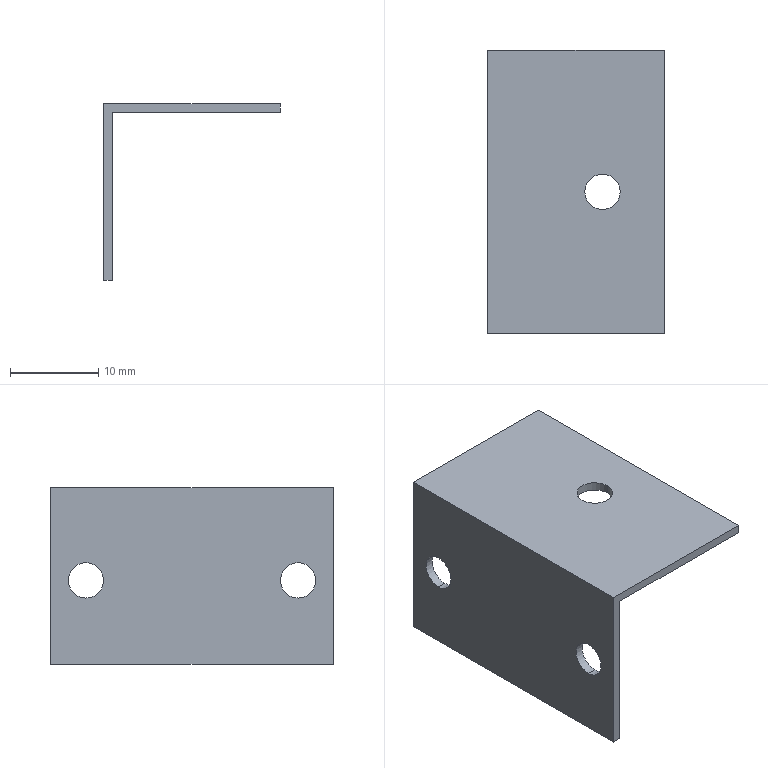Part | SolidWorks | features BaseBody 1 | 1 solid | 14 faces | box 20 x 32 x 20 mm | volume 1210 mm3 | plane 8 | cylinder 6 | commonest cylinder face diameters 4 x6
STEP:
#1=CARTESIAN_POINT('',(1.,16.,10.));
#2=VERTEX_POINT('',#1);
#3=CARTESIAN_POINT('',(5.,16.,10.));
#4=VERTEX_POINT('',#3);
#5=CARTESIAN_POINT('',(3.,16.,10.));
#6=DIRECTION('',(0.,0.,1.));
#7=DIRECTION('',(-1.,0.,0.));
#8=AXIS2_PLACEMENT_3D('',#5,#6,#7);
#9=CIRCLE('',#8,2.);
#10=EDGE_CURVE('',#2,#4,#9,.T.);
#11=ORIENTED_EDGE('',*,*,#10,.T.);
#12=CARTESIAN_POINT('',(5.,16.,9.));
#13=VERTEX_POINT('',#12);
#14=CARTESIAN_POINT('',(5.,16.,10.));
#15=DIRECTION('',(0.,0.,-1.));
#16=VECTOR('',#15,1000.);
#17=LINE('',#14,#16);
#18=EDGE_CURVE('',#4,#13,#17,.T.);
#19=ORIENTED_EDGE('',*,*,#18,.T.);
#20=CARTESIAN_POINT('',(1.,16.,9.));
#21=VERTEX_POINT('',#20);
#22=CARTESIAN_POINT('',(3.,16.,9.));
#23=DIRECTION('',(0.,0.,1.));
#24=DIRECTION('',(-1.,0.,0.));
#25=AXIS2_PLACEMENT_3D('',#22,#23,#24);
#26=CIRCLE('',#25,2.);
#27=EDGE_CURVE('',#21,#13,#26,.T.);
#28=ORIENTED_EDGE('',*,*,#27,.F.);
#29=CARTESIAN_POINT('',(1.,16.,10.));
#30=DIRECTION('',(0.,0.,-1.));
#31=VECTOR('',#30,1000.);
#32=LINE('',#29,#31);
#33=EDGE_CURVE('',#2,#21,#32,.T.);
#34=ORIENTED_EDGE('',*,*,#33,.F.);
#35=EDGE_LOOP('',(#11,#19,#28,#34));
#36=FACE_OUTER_BOUND('',#35,.T.);
#37=CARTESIAN_POINT('',(3.,16.,10.));
#38=DIRECTION('',(0.,0.,-1.));
#39=DIRECTION('',(-1.,0.,0.));
#40=AXIS2_PLACEMENT_3D('',#37,#38,#39);
#41=CYLINDRICAL_SURFACE('',#40,2.);
#42=ADVANCED_FACE('',(#36),#41,.F.);
#43=CARTESIAN_POINT('',(-10.,4.,1.5));
#44=VERTEX_POINT('',#43);
#45=CARTESIAN_POINT('',(-10.,4.,-2.5));
#46=VERTEX_POINT('',#45);
#47=CARTESIAN_POINT('',(-10.,4.,-0.5));
#48=DIRECTION('',(1.,0.,0.));
#49=DIRECTION('',(0.,0.,-1.));
#50=AXIS2_PLACEMENT_3D('',#47,#48,#49);
#51=CIRCLE('',#50,2.);
#52=EDGE_CURVE('',#44,#46,#51,.T.);
#53=ORIENTED_EDGE('',*,*,#52,.F.);
#54=CARTESIAN_POINT('',(-9.,4.,1.5));
#55=VERTEX_POINT('',#54);
#56=CARTESIAN_POINT('',(-29.,4.,1.5));
#57=DIRECTION('',(1.,0.,0.));
#58=VECTOR('',#57,1000.);
#59=LINE('',#56,#58);
#60=EDGE_CURVE('',#44,#55,#59,.T.);
#61=ORIENTED_EDGE('',*,*,#60,.T.);
#62=CARTESIAN_POINT('',(-9.,4.,-2.5));
#63=VERTEX_POINT('',#62);
#64=CARTESIAN_POINT('',(-9.,4.,-0.5));
#65=DIRECTION('',(-1.,0.,0.));
#66=DIRECTION('',(0.,0.,-1.));
#67=AXIS2_PLACEMENT_3D('',#64,#65,#66);
#68=CIRCLE('',#67,2.);
#69=EDGE_CURVE('',#63,#55,#68,.T.);
#70=ORIENTED_EDGE('',*,*,#69,.F.);
#71=CARTESIAN_POINT('',(-29.,4.,-2.5));
#72=DIRECTION('',(1.,0.,0.));
#73=VECTOR('',#72,1000.);
#74=LINE('',#71,#73);
#75=EDGE_CURVE('',#46,#63,#74,.T.);
#76=ORIENTED_EDGE('',*,*,#75,.F.);
#77=EDGE_LOOP('',(#53,#61,#70,#76));
#78=FACE_OUTER_BOUND('',#77,.T.);
#79=CARTESIAN_POINT('',(-29.,4.,-0.5));
#80=DIRECTION('',(1.,0.,0.));
#81=DIRECTION('',(0.,0.,-1.));
#82=AXIS2_PLACEMENT_3D('',#79,#80,#81);
#83=CYLINDRICAL_SURFACE('',#82,2.);
#84=ADVANCED_FACE('',(#78),#83,.F.);
#85=CARTESIAN_POINT('',(-10.,28.,1.5));
#86=VERTEX_POINT('',#85);
#87=CARTESIAN_POINT('',(-10.,28.,-2.5));
#88=VERTEX_POINT('',#87);
#89=CARTESIAN_POINT('',(-10.,28.,-0.5));
#90=DIRECTION('',(1.,0.,0.));
#91=DIRECTION('',(0.,0.,-1.));
#92=AXIS2_PLACEMENT_3D('',#89,#90,#91);
#93=CIRCLE('',#92,2.);
#94=EDGE_CURVE('',#86,#88,#93,.T.);
#95=ORIENTED_EDGE('',*,*,#94,.F.);
#96=CARTESIAN_POINT('',(-9.,28.,1.5));
#97=VERTEX_POINT('',#96);
#98=CARTESIAN_POINT('',(-29.,28.,1.5));
#99=DIRECTION('',(1.,0.,0.));
#100=VECTOR('',#99,1000.);
#101=LINE('',#98,#100);
#102=EDGE_CURVE('',#86,#97,#101,.T.);
#103=ORIENTED_EDGE('',*,*,#102,.T.);
#104=CARTESIAN_POINT('',(-9.,28.,-2.5));
#105=VERTEX_POINT('',#104);
#106=CARTESIAN_POINT('',(-9.,28.,-0.5));
#107=DIRECTION('',(-1.,0.,0.));
#108=DIRECTION('',(0.,0.,-1.));
#109=AXIS2_PLACEMENT_3D('',#106,#107,#108);
#110=CIRCLE('',#109,2.);
#111=EDGE_CURVE('',#105,#97,#110,.T.);
#112=ORIENTED_EDGE('',*,*,#111,.F.);
#113=CARTESIAN_POINT('',(-29.,28.,-2.5));
#114=DIRECTION('',(1.,0.,0.));
#115=VECTOR('',#114,1000.);
#116=LINE('',#113,#115);
#117=EDGE_CURVE('',#88,#105,#116,.T.);
#118=ORIENTED_EDGE('',*,*,#117,.F.);
#119=EDGE_LOOP('',(#95,#103,#112,#118));
#120=FACE_OUTER_BOUND('',#119,.T.);
#121=CARTESIAN_POINT('',(-29.,28.,-0.5));
#122=DIRECTION('',(1.,0.,0.));
#123=DIRECTION('',(0.,0.,-1.));
#124=AXIS2_PLACEMENT_3D('',#121,#122,#123);
#125=CYLINDRICAL_SURFACE('',#124,2.);
#126=ADVANCED_FACE('',(#120),#125,.F.);
#127=CARTESIAN_POINT('',(10.,32.,10.));
#128=VERTEX_POINT('',#127);
#129=CARTESIAN_POINT('',(10.,0.,10.));
#130=VERTEX_POINT('',#129);
#131=CARTESIAN_POINT('',(10.,32.,10.));
#132=DIRECTION('',(0.,-1.,0.));
#133=VECTOR('',#132,1000.);
#134=LINE('',#131,#133);
#135=EDGE_CURVE('',#128,#130,#134,.T.);
#136=ORIENTED_EDGE('',*,*,#135,.F.);
#137=CARTESIAN_POINT('',(-10.,32.,10.));
#138=VERTEX_POINT('',#137);
#139=CARTESIAN_POINT('',(0.,32.,10.));
#140=DIRECTION('',(1.,0.,0.));
#141=VECTOR('',#140,1000.);
#142=LINE('',#139,#141);
#143=EDGE_CURVE('',#138,#128,#142,.T.);
#144=ORIENTED_EDGE('',*,*,#143,.F.);
#145=CARTESIAN_POINT('',(-10.,0.,10.));
#146=VERTEX_POINT('',#145);
#147=CARTESIAN_POINT('',(-10.,32.,10.));
#148=DIRECTION('',(0.,1.,0.));
#149=VECTOR('',#148,1000.);
#150=LINE('',#147,#149);
#151=EDGE_CURVE('',#146,#138,#150,.T.);
#152=ORIENTED_EDGE('',*,*,#151,.F.);
#153=CARTESIAN_POINT('',(0.,0.,10.));
#154=DIRECTION('',(-1.,0.,0.));
#155=VECTOR('',#154,1000.);
#156=LINE('',#153,#155);
#157=EDGE_CURVE('',#130,#146,#156,.T.);
#158=ORIENTED_EDGE('',*,*,#157,.F.);
#159=EDGE_LOOP('',(#136,#144,#152,#158));
#160=FACE_OUTER_BOUND('',#159,.T.);
#161=ORIENTED_EDGE('',*,*,#10,.F.);
#162=CARTESIAN_POINT('',(3.,16.,10.));
#163=DIRECTION('',(0.,0.,1.));
#164=DIRECTION('',(-1.,0.,0.));
#165=AXIS2_PLACEMENT_3D('',#162,#163,#164);
#166=CIRCLE('',#165,2.);
#167=EDGE_CURVE('',#4,#2,#166,.T.);
#168=ORIENTED_EDGE('',*,*,#167,.F.);
#169=EDGE_LOOP('',(#161,#168));
#170=FACE_BOUND('',#169,.T.);
#171=CARTESIAN_POINT('',(0.,32.,10.));
#172=DIRECTION('',(0.,0.,-1.));
#173=DIRECTION('',(-1.,0.,0.));
#174=AXIS2_PLACEMENT_3D('',#171,#172,#173);
#175=PLANE('',#174);
#176=ADVANCED_FACE('',(#160,#170),#175,.F.);
#177=CARTESIAN_POINT('',(10.,0.,9.));
#178=VERTEX_POINT('',#177);
#179=CARTESIAN_POINT('',(-9.,0.,9.));
#180=VERTEX_POINT('',#179);
#181=CARTESIAN_POINT('',(0.,0.,9.));
#182=DIRECTION('',(-1.,0.,0.));
#183=VECTOR('',#182,1000.);
#184=LINE('',#181,#183);
#185=EDGE_CURVE('',#178,#180,#184,.T.);
#186=ORIENTED_EDGE('',*,*,#185,.F.);
#187=CARTESIAN_POINT('',(10.,0.,0.));
#188=DIRECTION('',(0.,0.,-1.));
#189=VECTOR('',#188,1000.);
#190=LINE('',#187,#189);
#191=EDGE_CURVE('',#130,#178,#190,.T.);
#192=ORIENTED_EDGE('',*,*,#191,.F.);
#193=ORIENTED_EDGE('',*,*,#157,.T.);
#194=CARTESIAN_POINT('',(-10.,0.,-10.));
#195=VERTEX_POINT('',#194);
#196=CARTESIAN_POINT('',(-10.,0.,0.));
#197=DIRECTION('',(0.,0.,1.));
#198=VECTOR('',#197,1000.);
#199=LINE('',#196,#198);
#200=EDGE_CURVE('',#195,#146,#199,.T.);
#201=ORIENTED_EDGE('',*,*,#200,.F.);
#202=CARTESIAN_POINT('',(-9.,0.,-10.));
#203=VERTEX_POINT('',#202);
#204=CARTESIAN_POINT('',(0.,0.,-10.));
#205=DIRECTION('',(-1.,0.,0.));
#206=VECTOR('',#205,1000.);
#207=LINE('',#204,#206);
#208=EDGE_CURVE('',#203,#195,#207,.T.);
#209=ORIENTED_EDGE('',*,*,#208,.F.);
#210=CARTESIAN_POINT('',(-9.,0.,0.));
#211=DIRECTION('',(0.,0.,-1.));
#212=VECTOR('',#211,1000.);
#213=LINE('',#210,#212);
#214=EDGE_CURVE('',#180,#203,#213,.T.);
#215=ORIENTED_EDGE('',*,*,#214,.F.);
#216=EDGE_LOOP('',(#186,#192,#193,#201,#209,#215));
#217=FACE_OUTER_BOUND('',#216,.T.);
#218=CARTESIAN_POINT('',(0.,0.,0.));
#219=DIRECTION('',(0.,1.,0.));
#220=DIRECTION('',(0.,0.,1.));
#221=AXIS2_PLACEMENT_3D('',#218,#219,#220);
#222=PLANE('',#221);
#223=ADVANCED_FACE('',(#217),#222,.F.);
#224=CARTESIAN_POINT('',(10.,32.,9.));
#225=VERTEX_POINT('',#224);
#226=CARTESIAN_POINT('',(10.,32.,9.));
#227=DIRECTION('',(0.,-1.,0.));
#228=VECTOR('',#227,1000.);
#229=LINE('',#226,#228);
#230=EDGE_CURVE('',#225,#178,#229,.T.);
#231=ORIENTED_EDGE('',*,*,#230,.F.);
#232=CARTESIAN_POINT('',(10.,32.,0.));
#233=DIRECTION('',(0.,0.,-1.));
#234=VECTOR('',#233,1000.);
#235=LINE('',#232,#234);
#236=EDGE_CURVE('',#128,#225,#235,.T.);
#237=ORIENTED_EDGE('',*,*,#236,.F.);
#238=ORIENTED_EDGE('',*,*,#135,.T.);
#239=ORIENTED_EDGE('',*,*,#191,.T.);
#240=EDGE_LOOP('',(#231,#237,#238,#239));
#241=FACE_OUTER_BOUND('',#240,.T.);
#242=CARTESIAN_POINT('',(10.,32.,0.));
#243=DIRECTION('',(-1.,0.,0.));
#244=DIRECTION('',(0.,0.,1.));
#245=AXIS2_PLACEMENT_3D('',#242,#243,#244);
#246=PLANE('',#245);
#247=ADVANCED_FACE('',(#241),#246,.F.);
#248=ORIENTED_EDGE('',*,*,#236,.T.);
#249=CARTESIAN_POINT('',(-9.,32.,9.));
#250=VERTEX_POINT('',#249);
#251=CARTESIAN_POINT('',(0.,32.,9.));
#252=DIRECTION('',(-1.,0.,0.));
#253=VECTOR('',#252,1000.);
#254=LINE('',#251,#253);
#255=EDGE_CURVE('',#225,#250,#254,.T.);
#256=ORIENTED_EDGE('',*,*,#255,.T.);
#257=CARTESIAN_POINT('',(-9.,32.,-10.));
#258=VERTEX_POINT('',#257);
#259=CARTESIAN_POINT('',(-9.,32.,0.));
#260=DIRECTION('',(0.,0.,-1.));
#261=VECTOR('',#260,1000.);
#262=LINE('',#259,#261);
#263=EDGE_CURVE('',#250,#258,#262,.T.);
#264=ORIENTED_EDGE('',*,*,#263,.T.);
#265=CARTESIAN_POINT('',(-10.,32.,-10.));
#266=VERTEX_POINT('',#265);
#267=CARTESIAN_POINT('',(0.,32.,-10.));
#268=DIRECTION('',(1.,0.,0.));
#269=VECTOR('',#268,1000.);
#270=LINE('',#267,#269);
#271=EDGE_CURVE('',#266,#258,#270,.T.);
#272=ORIENTED_EDGE('',*,*,#271,.F.);
#273=CARTESIAN_POINT('',(-10.,32.,0.));
#274=DIRECTION('',(0.,0.,1.));
#275=VECTOR('',#274,1000.);
#276=LINE('',#273,#275);
#277=EDGE_CURVE('',#266,#138,#276,.T.);
#278=ORIENTED_EDGE('',*,*,#277,.T.);
#279=ORIENTED_EDGE('',*,*,#143,.T.);
#280=EDGE_LOOP('',(#248,#256,#264,#272,#278,#279));
#281=FACE_OUTER_BOUND('',#280,.T.);
#282=CARTESIAN_POINT('',(0.,32.,0.));
#283=DIRECTION('',(0.,1.,0.));
#284=DIRECTION('',(0.,0.,1.));
#285=AXIS2_PLACEMENT_3D('',#282,#283,#284);
#286=PLANE('',#285);
#287=ADVANCED_FACE('',(#281),#286,.T.);
#288=ORIENTED_EDGE('',*,*,#277,.F.);
#289=CARTESIAN_POINT('',(-10.,32.,-10.));
#290=DIRECTION('',(0.,-1.,0.));
#291=VECTOR('',#290,1000.);
#292=LINE('',#289,#291);
#293=EDGE_CURVE('',#266,#195,#292,.T.);
#294=ORIENTED_EDGE('',*,*,#293,.T.);
#295=ORIENTED_EDGE('',*,*,#200,.T.);
#296=ORIENTED_EDGE('',*,*,#151,.T.);
#297=EDGE_LOOP('',(#288,#294,#295,#296));
#298=FACE_OUTER_BOUND('',#297,.T.);
#299=CARTESIAN_POINT('',(-10.,4.,-0.5));
#300=DIRECTION('',(1.,0.,0.));
#301=DIRECTION('',(0.,0.,-1.));
#302=AXIS2_PLACEMENT_3D('',#299,#300,#301);
#303=CIRCLE('',#302,2.);
#304=EDGE_CURVE('',#46,#44,#303,.T.);
#305=ORIENTED_EDGE('',*,*,#304,.T.);
#306=ORIENTED_EDGE('',*,*,#52,.T.);
#307=EDGE_LOOP('',(#305,#306));
#308=FACE_BOUND('',#307,.T.);
#309=CARTESIAN_POINT('',(-10.,28.,-0.5));
#310=DIRECTION('',(1.,0.,0.));
#311=DIRECTION('',(0.,0.,-1.));
#312=AXIS2_PLACEMENT_3D('',#309,#310,#311);
#313=CIRCLE('',#312,2.);
#314=EDGE_CURVE('',#88,#86,#313,.T.);
#315=ORIENTED_EDGE('',*,*,#314,.T.);
#316=ORIENTED_EDGE('',*,*,#94,.T.);
#317=EDGE_LOOP('',(#315,#316));
#318=FACE_BOUND('',#317,.T.);
#319=CARTESIAN_POINT('',(-10.,32.,0.));
#320=DIRECTION('',(-1.,0.,0.));
#321=DIRECTION('',(0.,0.,1.));
#322=AXIS2_PLACEMENT_3D('',#319,#320,#321);
#323=PLANE('',#322);
#324=ADVANCED_FACE('',(#298,#308,#318),#323,.T.);
#325=ORIENTED_EDGE('',*,*,#18,.F.);
#326=ORIENTED_EDGE('',*,*,#167,.T.);
#327=ORIENTED_EDGE('',*,*,#33,.T.);
#328=CARTESIAN_POINT('',(3.,16.,9.));
#329=DIRECTION('',(0.,0.,1.));
#330=DIRECTION('',(-1.,0.,0.));
#331=AXIS2_PLACEMENT_3D('',#328,#329,#330);
#332=CIRCLE('',#331,2.);
#333=EDGE_CURVE('',#13,#21,#332,.T.);
#334=ORIENTED_EDGE('',*,*,#333,.F.);
#335=EDGE_LOOP('',(#325,#326,#327,#334));
#336=FACE_OUTER_BOUND('',#335,.T.);
#337=CARTESIAN_POINT('',(3.,16.,10.));
#338=DIRECTION('',(0.,0.,-1.));
#339=DIRECTION('',(-1.,0.,0.));
#340=AXIS2_PLACEMENT_3D('',#337,#338,#339);
#341=CYLINDRICAL_SURFACE('',#340,2.);
#342=ADVANCED_FACE('',(#336),#341,.F.);
#343=ORIENTED_EDGE('',*,*,#263,.F.);
#344=CARTESIAN_POINT('',(-9.,32.,9.));
#345=DIRECTION('',(0.,-1.,0.));
#346=VECTOR('',#345,1000.);
#347=LINE('',#344,#346);
#348=EDGE_CURVE('',#250,#180,#347,.T.);
#349=ORIENTED_EDGE('',*,*,#348,.T.);
#350=ORIENTED_EDGE('',*,*,#214,.T.);
#351=CARTESIAN_POINT('',(-9.,32.,-10.));
#352=DIRECTION('',(0.,1.,0.));
#353=VECTOR('',#352,1000.);
#354=LINE('',#351,#353);
#355=EDGE_CURVE('',#203,#258,#354,.T.);
#356=ORIENTED_EDGE('',*,*,#355,.T.);
#357=EDGE_LOOP('',(#343,#349,#350,#356));
#358=FACE_OUTER_BOUND('',#357,.T.);
#359=ORIENTED_EDGE('',*,*,#69,.T.);
#360=CARTESIAN_POINT('',(-9.,4.,-0.5));
#361=DIRECTION('',(-1.,0.,0.));
#362=DIRECTION('',(0.,0.,-1.));
#363=AXIS2_PLACEMENT_3D('',#360,#361,#362);
#364=CIRCLE('',#363,2.);
#365=EDGE_CURVE('',#55,#63,#364,.T.);
#366=ORIENTED_EDGE('',*,*,#365,.T.);
#367=EDGE_LOOP('',(#359,#366));
#368=FACE_BOUND('',#367,.T.);
#369=ORIENTED_EDGE('',*,*,#111,.T.);
#370=CARTESIAN_POINT('',(-9.,28.,-0.5));
#371=DIRECTION('',(-1.,0.,0.));
#372=DIRECTION('',(0.,0.,-1.));
#373=AXIS2_PLACEMENT_3D('',#370,#371,#372);
#374=CIRCLE('',#373,2.);
#375=EDGE_CURVE('',#97,#105,#374,.T.);
#376=ORIENTED_EDGE('',*,*,#375,.T.);
#377=EDGE_LOOP('',(#369,#376));
#378=FACE_BOUND('',#377,.T.);
#379=CARTESIAN_POINT('',(-9.,32.,0.));
#380=DIRECTION('',(1.,0.,0.));
#381=DIRECTION('',(0.,0.,-1.));
#382=AXIS2_PLACEMENT_3D('',#379,#380,#381);
#383=PLANE('',#382);
#384=ADVANCED_FACE('',(#358,#368,#378),#383,.T.);
#385=ORIENTED_EDGE('',*,*,#348,.F.);
#386=ORIENTED_EDGE('',*,*,#255,.F.);
#387=ORIENTED_EDGE('',*,*,#230,.T.);
#388=ORIENTED_EDGE('',*,*,#185,.T.);
#389=EDGE_LOOP('',(#385,#386,#387,#388));
#390=FACE_OUTER_BOUND('',#389,.T.);
#391=ORIENTED_EDGE('',*,*,#27,.T.);
#392=ORIENTED_EDGE('',*,*,#333,.T.);
#393=EDGE_LOOP('',(#391,#392));
#394=FACE_BOUND('',#393,.T.);
#395=CARTESIAN_POINT('',(0.,32.,9.));
#396=DIRECTION('',(0.,0.,1.));
#397=DIRECTION('',(1.,0.,0.));
#398=AXIS2_PLACEMENT_3D('',#395,#396,#397);
#399=PLANE('',#398);
#400=ADVANCED_FACE('',(#390,#394),#399,.F.);
#401=ORIENTED_EDGE('',*,*,#271,.T.);
#402=ORIENTED_EDGE('',*,*,#355,.F.);
#403=ORIENTED_EDGE('',*,*,#208,.T.);
#404=ORIENTED_EDGE('',*,*,#293,.F.);
#405=EDGE_LOOP('',(#401,#402,#403,#404));
#406=FACE_OUTER_BOUND('',#405,.T.);
#407=CARTESIAN_POINT('',(0.,32.,-10.));
#408=DIRECTION('',(0.,0.,-1.));
#409=DIRECTION('',(-1.,0.,0.));
#410=AXIS2_PLACEMENT_3D('',#407,#408,#409);
#411=PLANE('',#410);
#412=ADVANCED_FACE('',(#406),#411,.T.);
#413=ORIENTED_EDGE('',*,*,#60,.F.);
#414=ORIENTED_EDGE('',*,*,#304,.F.);
#415=ORIENTED_EDGE('',*,*,#75,.T.);
#416=ORIENTED_EDGE('',*,*,#365,.F.);
#417=EDGE_LOOP('',(#413,#414,#415,#416));
#418=FACE_OUTER_BOUND('',#417,.T.);
#419=CARTESIAN_POINT('',(-29.,4.,-0.5));
#420=DIRECTION('',(1.,0.,0.));
#421=DIRECTION('',(0.,0.,-1.));
#422=AXIS2_PLACEMENT_3D('',#419,#420,#421);
#423=CYLINDRICAL_SURFACE('',#422,2.);
#424=ADVANCED_FACE('',(#418),#423,.F.);
#425=ORIENTED_EDGE('',*,*,#102,.F.);
#426=ORIENTED_EDGE('',*,*,#314,.F.);
#427=ORIENTED_EDGE('',*,*,#117,.T.);
#428=ORIENTED_EDGE('',*,*,#375,.F.);
#429=EDGE_LOOP('',(#425,#426,#427,#428));
#430=FACE_OUTER_BOUND('',#429,.T.);
#431=CARTESIAN_POINT('',(-29.,28.,-0.5));
#432=DIRECTION('',(1.,0.,0.));
#433=DIRECTION('',(0.,0.,-1.));
#434=AXIS2_PLACEMENT_3D('',#431,#432,#433);
#435=CYLINDRICAL_SURFACE('',#434,2.);
#436=ADVANCED_FACE('',(#430),#435,.F.);
#437=CLOSED_SHELL('',(#42,#84,#126,#176,#223,#247,#287,#324,#342,#384,#400,#412,#424,#436));
#438=MANIFOLD_SOLID_BREP('',#437);
#439=CARTESIAN_POINT('',(0.,0.,0.));
#440=DIRECTION('',(0.,0.,1.));
#441=DIRECTION('',(1.,0.,0.));
#442=AXIS2_PLACEMENT_3D('',#439,#440,#441);
#443=(LENGTH_UNIT()NAMED_UNIT(*)SI_UNIT(.MILLI.,.METRE.));
#444=UNCERTAINTY_MEASURE_WITH_UNIT(LENGTH_MEASURE(0.00001),#443,'','');
#445=(NAMED_UNIT(*)PLANE_ANGLE_UNIT()SI_UNIT($,.RADIAN.));
#446=(NAMED_UNIT(*)SI_UNIT($,.STERADIAN.)SOLID_ANGLE_UNIT());
#447=(GEOMETRIC_REPRESENTATION_CONTEXT(3)GLOBAL_UNCERTAINTY_ASSIGNED_CONTEXT((#444))GLOBAL_UNIT_ASSIGNED_CONTEXT((#443,#445,#446))REPRESENTATION_CONTEXT('',''));
#448=ADVANCED_BREP_SHAPE_REPRESENTATION('',(#438,#442),#447);